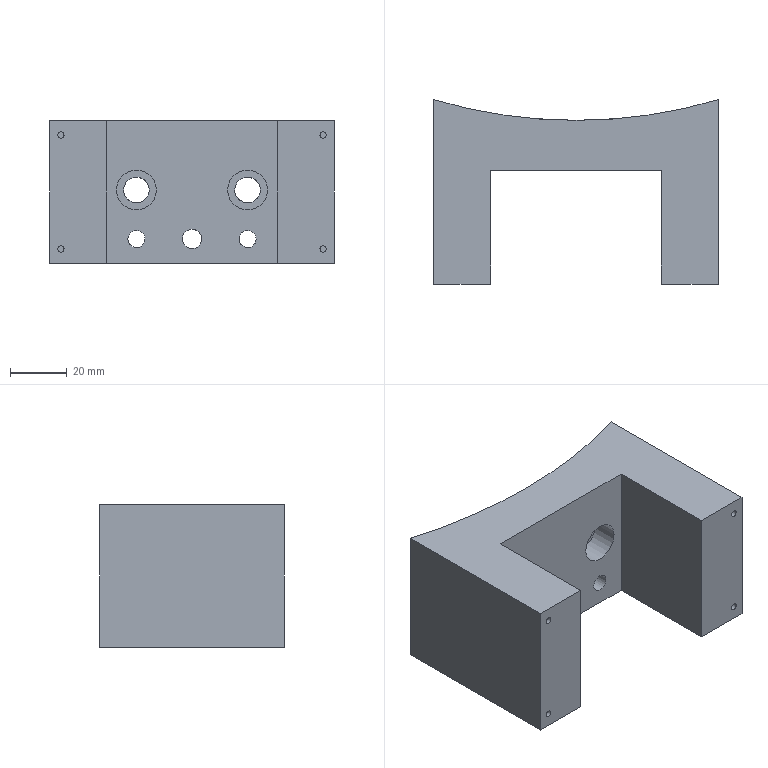NC program | NX | posted with a generic post | part box 100 x 64.77 x 50 mm
Lines 1 to 978 of 7818:
N10 G17 G21 G94 G90
(ZLEVEL_PROFILE_1 , TOOL : D50R0.8)
N12 T02 M6
N14 G54
N16 G17 G0 G90 X2.648 Y76.918 B0. C0. S1200 M3
N18 G43 Z30. H2
N20 Z7.002
N22 G94 G1 X2.631 Y76.907 Z6.512 F1500.
N24 X2.581 Y76.87 Z6.043
N26 X2.501 Y76.808 Z5.594
N28 X2.391 Y76.72 Z5.164
N30 X2.254 Y76.602 Z4.754
N32 X2.093 Y76.455 Z4.363
N34 X1.908 Y76.278 Z3.99
N36 X1.702 Y76.068 Z3.636
N38 X1.476 Y75.825 Z3.299
N40 X1.234 Y75.547 Z2.979
N42 X0.976 Y75.233 Z2.677
N44 X0.704 Y74.881 Z2.391
N46 X0.421 Y74.492 Z2.121
N48 X0.128 Y74.062 Z1.867
N50 X-0.173 Y73.591 Z1.629
N52 X-0.479 Y73.078 Z1.405
N54 X-0.789 Y72.52 Z1.196
N56 X-1.102 Y71.918 Z1.002
N58 X-1.414 Y71.27 Z0.821
N60 X-1.724 Y70.574 Z0.654
N62 X-2.03 Y69.829 Z0.5
N64 X-2.331 Y69.034 Z0.359
N66 X-2.624 Y68.188 Z0.23
N68 X-2.907 Y67.289 Z0.113
N70 X-3.179 Y66.336 Z0.008
N72 X-3.437 Y65.327 Z-0.087
N74 X-3.679 Y64.262 Z-0.17
N76 X-3.905 Y63.139 Z-0.243
N78 X-4.111 Y61.957 Z-0.306
N80 X-4.296 Y60.715 Z-0.359
N82 X-4.457 Y59.41 Z-0.403
N84 X-4.594 Y58.043 Z-0.438
N86 X-4.704 Y56.612 Z-0.465
N88 X-4.784 Y55.115 Z-0.484
N90 X-4.834 Y53.551 Z-0.495
N92 X-4.851 Y51.918 Z-0.498
N94 X-4.85 Y22.992
N96 Y-25.
N98 X-4.851 Y-51.918
N100 X-4.835 Y-52.334
N102 X-4.788 Y-52.725
N104 X-4.714 Y-53.093
N106 X-4.613 Y-53.437
N108 X-4.488 Y-53.759
N110 X-4.341 Y-54.06
N112 X-4.175 Y-54.34
N114 X-3.991 Y-54.6
N116 X-3.792 Y-54.841
N118 X-3.58 Y-55.064
N120 X-3.358 Y-55.268
N122 X-3.127 Y-55.456
N124 X-2.889 Y-55.627
N126 X-2.648 Y-55.782
N128 X-2.404 Y-55.923
N130 X-2.161 Y-56.05
N132 X-1.92 Y-56.163
N134 X-1.52 Y-56.327
N136 X-1.13 Y-56.455
N138 X-0.749 Y-56.546
N140 X-0.373 Y-56.6
N142 X0.001 Y-56.618
N144 X0.374 Y-56.6
N146 X0.75 Y-56.546
N148 X1.132 Y-56.455
N150 X1.521 Y-56.327
N152 X1.921 Y-56.163
N154 X2.162 Y-56.05
N156 X2.405 Y-55.923
N158 X2.649 Y-55.782
N160 X2.891 Y-55.627
N162 X3.128 Y-55.456
N164 X3.359 Y-55.268
N166 X3.582 Y-55.064
N168 X3.793 Y-54.841
N170 X3.992 Y-54.6
N172 X4.176 Y-54.34
N174 X4.342 Y-54.06
N176 X4.489 Y-53.759
N178 X4.614 Y-53.437
N180 X4.715 Y-53.093
N182 X4.79 Y-52.725
N184 X4.836 Y-52.334
N186 X4.852 Y-51.918
N188 Y-25.76
N190 X4.85 Y-25.006
N192 Y22.992
N194 X4.852 Y51.918
N196 X4.836 Y52.335 Z-0.499
N198 X4.79 Y52.726 Z-0.501
N200 X4.715 Y53.094 Z-0.504
N202 X4.614 Y53.439 Z-0.508
N204 X4.489 Y53.762 Z-0.513
N206 X4.342 Y54.063 Z-0.519
N208 X4.176 Y54.344 Z-0.526
N210 X3.992 Y54.604 Z-0.534
N212 X3.793 Y54.846 Z-0.543
N214 X3.581 Y55.068 Z-0.552
N216 X3.359 Y55.273 Z-0.562
N218 X3.128 Y55.461 Z-0.573
N220 X2.89 Y55.633 Z-0.584
N222 X2.649 Y55.789 Z-0.596
N224 X2.405 Y55.93 Z-0.608
N226 X2.162 Y56.057 Z-0.62
N228 X1.921 Y56.171 Z-0.633
N230 X1.521 Y56.335 Z-0.655
N232 X1.131 Y56.463 Z-0.678
N234 X0.75 Y56.555 Z-0.701
N236 X0.374 Y56.61 Z-0.724
N238 X0.001 Y56.628 Z-0.747
N240 X-0.373 Y56.61 Z-0.771
N242 X-0.749 Y56.556 Z-0.794
N244 X-1.13 Y56.465 Z-0.817
N246 X-1.519 Y56.338 Z-0.839
N248 X-1.919 Y56.174 Z-0.861
N250 X-2.16 Y56.061 Z-0.874
N252 X-2.404 Y55.934 Z-0.886
N254 X-2.647 Y55.793 Z-0.899
N256 X-2.889 Y55.638 Z-0.91
N258 X-3.127 Y55.466 Z-0.921
N260 X-3.358 Y55.279 Z-0.932
N262 X-3.58 Y55.074 Z-0.942
N264 X-3.792 Y54.852 Z-0.952
N266 X-3.991 Y54.611 Z-0.96
N268 X-4.174 Y54.35 Z-0.968
N270 X-4.341 Y54.07 Z-0.975
N272 X-4.488 Y53.769 Z-0.981
N274 X-4.612 Y53.446 Z-0.987
N276 X-4.714 Y53.101 Z-0.991
N278 X-4.788 Y52.734 Z-0.994
N280 X-4.835 Y52.342 Z-0.996
N282 X-4.851 Y51.926
N284 X-4.85 Y24.701
N286 Y-25.
N288 X-4.851 Y-51.926
N290 X-4.835 Y-52.341
N292 X-4.788 Y-52.732
N294 X-4.713 Y-53.1
N296 X-4.612 Y-53.444
N298 X-4.487 Y-53.767
N300 X-4.34 Y-54.068
N302 X-4.174 Y-54.348
N304 X-3.99 Y-54.608
N306 X-3.791 Y-54.849
N308 X-3.579 Y-55.071
N310 X-3.356 Y-55.275
N312 X-3.125 Y-55.463
N314 X-2.887 Y-55.634
N316 X-2.645 Y-55.79
N318 X-2.401 Y-55.931
N320 X-2.157 Y-56.057
N322 X-1.916 Y-56.171
N324 X-1.515 Y-56.335
N326 X-1.125 Y-56.462
N328 X-0.743 Y-56.553
N330 X-0.367 Y-56.607
N332 X0.007 Y-56.626
N334 X0.381 Y-56.607
N336 X0.758 Y-56.553
N338 X1.14 Y-56.462
N340 X1.529 Y-56.335
N342 X1.93 Y-56.171
N344 X2.171 Y-56.057
N346 X2.414 Y-55.931
N348 X2.657 Y-55.79
N350 X2.899 Y-55.634
N352 X3.136 Y-55.463
N354 X3.367 Y-55.275
N356 X3.589 Y-55.071
N358 X3.801 Y-54.849
N360 X3.999 Y-54.608
N362 X4.182 Y-54.348
N364 X4.348 Y-54.068
N366 X4.494 Y-53.767
N368 X4.618 Y-53.444
N370 X4.718 Y-53.1
N372 X4.792 Y-52.732
N374 X4.837 Y-52.341
N376 X4.852 Y-51.926
N378 X4.851 Y-51.519
N380 Y-26.035
N382 X4.85 Y-25.
N384 Y24.701
N386 X4.852 Y51.926
N388 X4.836 Y52.342 Z-0.997
N390 X4.79 Y52.734 Z-0.999
N392 X4.715 Y53.102 Z-1.002
N394 X4.614 Y53.447 Z-1.006
N396 X4.489 Y53.769 Z-1.011
N398 X4.342 Y54.071 Z-1.017
N400 X4.176 Y54.351 Z-1.024
N402 X3.992 Y54.612 Z-1.032
N404 X3.793 Y54.853 Z-1.041
N406 X3.581 Y55.076 Z-1.05
N408 X3.359 Y55.281 Z-1.06
N410 X3.128 Y55.469 Z-1.071
N412 X2.89 Y55.64 Z-1.082
N414 X2.649 Y55.796 Z-1.094
N416 X2.405 Y55.937 Z-1.106
N418 X2.162 Y56.065 Z-1.118
N420 X1.921 Y56.178 Z-1.131
N422 X1.521 Y56.343 Z-1.153
N424 X1.131 Y56.47 Z-1.176
N426 X0.75 Y56.562 Z-1.199
N428 X0.374 Y56.617 Z-1.222
N430 X0.001 Y56.635 Z-1.245
N432 X-0.373 Y56.618 Z-1.269
N434 X-0.749 Y56.563 Z-1.292
N436 X-1.13 Y56.473 Z-1.315
N438 X-1.519 Y56.345 Z-1.337
N440 X-1.919 Y56.182 Z-1.359
N442 X-2.16 Y56.068 Z-1.372
N444 X-2.404 Y55.942 Z-1.385
N446 X-2.647 Y55.801 Z-1.397
N448 X-2.889 Y55.645 Z-1.408
N450 X-3.127 Y55.474 Z-1.42
N452 X-3.358 Y55.286 Z-1.43
N454 X-3.58 Y55.082 Z-1.44
N456 X-3.792 Y54.859 Z-1.45
N458 X-3.991 Y54.618 Z-1.458
N460 X-4.174 Y54.358 Z-1.466
N462 X-4.341 Y54.077 Z-1.473
N464 X-4.488 Y53.776 Z-1.48
N466 X-4.613 Y53.454 Z-1.485
N468 X-4.714 Y53.109 Z-1.489
N470 X-4.788 Y52.741 Z-1.492
N472 X-4.835 Y52.349 Z-1.494
N474 X-4.851 Y51.933
N476 X-4.85 Y24.701
N478 Y-25.
N480 X-4.851 Y-51.933
N482 X-4.835 Y-52.349
N484 X-4.788 Y-52.74
N486 X-4.713 Y-53.107
N488 X-4.612 Y-53.452
N490 X-4.487 Y-53.774
N492 X-4.34 Y-54.075
N494 X-4.174 Y-54.355
N496 X-3.99 Y-54.615
N498 X-3.791 Y-54.856
N500 X-3.579 Y-55.078
N502 X-3.356 Y-55.283
N504 X-3.125 Y-55.47
N506 X-2.887 Y-55.641
N508 X-2.645 Y-55.797
N510 X-2.401 Y-55.938
N512 X-2.157 Y-56.065
N514 X-1.916 Y-56.178
N516 X-1.515 Y-56.342
N518 X-1.125 Y-56.469
N520 X-0.743 Y-56.56
N522 X-0.367 Y-56.615
N524 X0.007 Y-56.633
N526 X0.381 Y-56.615
N528 X0.758 Y-56.56
N530 X1.14 Y-56.469
N532 X1.529 Y-56.342
N534 X1.93 Y-56.178
N536 X2.171 Y-56.065
N538 X2.414 Y-55.938
N540 X2.657 Y-55.797
N542 X2.899 Y-55.641
N544 X3.136 Y-55.47
N546 X3.367 Y-55.283
N548 X3.589 Y-55.078
N550 X3.801 Y-54.856
N552 X3.999 Y-54.615
N554 X4.182 Y-54.355
N556 X4.348 Y-54.075
N558 X4.494 Y-53.774
N560 X4.618 Y-53.452
N562 X4.718 Y-53.107
N564 X4.792 Y-52.74
N566 X4.837 Y-52.349
N568 X4.852 Y-51.933
N570 X4.851 Y-51.519
N572 Y-26.035
N574 X4.85 Y-25.
N576 Y24.701
N578 X4.852 Y51.933
N580 X4.836 Y52.349 Z-1.495
N582 X4.79 Y52.741 Z-1.497
N584 X4.715 Y53.109 Z-1.5
N586 X4.614 Y53.454 Z-1.504
N588 X4.489 Y53.777 Z-1.509
N590 X4.342 Y54.078 Z-1.515
N592 X4.176 Y54.359 Z-1.522
N594 X3.992 Y54.619 Z-1.53
N596 X3.793 Y54.86 Z-1.539
N598 X3.581 Y55.083 Z-1.548
N600 X3.359 Y55.288 Z-1.559
N602 X3.128 Y55.476 Z-1.569
N604 X2.89 Y55.648 Z-1.58
N606 X2.649 Y55.804 Z-1.592
N608 X2.405 Y55.945 Z-1.604
N610 X2.162 Y56.072 Z-1.617
N612 X1.921 Y56.186 Z-1.629
N614 X1.521 Y56.35 Z-1.651
N616 X1.131 Y56.478 Z-1.674
N618 X0.75 Y56.569 Z-1.697
N620 X0.374 Y56.624 Z-1.72
N622 X0.001 Y56.643 Z-1.743
N624 X-0.373 Y56.625 Z-1.767
N626 X-0.749 Y56.571 Z-1.79
N628 X-1.13 Y56.48 Z-1.813
N630 X-1.519 Y56.353 Z-1.836
N632 X-1.919 Y56.189 Z-1.858
N634 X-2.16 Y56.076 Z-1.87
N636 X-2.404 Y55.949 Z-1.883
N638 X-2.647 Y55.808 Z-1.895
N640 X-2.889 Y55.652 Z-1.906
N642 X-3.127 Y55.481 Z-1.918
N644 X-3.358 Y55.294 Z-1.928
N646 X-3.58 Y55.089 Z-1.938
N648 X-3.792 Y54.866 Z-1.948
N650 X-3.991 Y54.625 Z-1.957
N652 X-4.174 Y54.365 Z-1.964
N654 X-4.341 Y54.085 Z-1.972
N656 X-4.488 Y53.784 Z-1.978
N658 X-4.613 Y53.461 Z-1.983
N660 X-4.714 Y53.116 Z-1.987
N662 X-4.788 Y52.748 Z-1.99
N664 X-4.835 Y52.357 Z-1.992
N666 X-4.851 Y51.94 Z-1.993
N668 X-4.85 Y24.701
N670 Y-25.
N672 X-4.851 Y-51.94
N674 X-4.835 Y-52.356
N676 X-4.788 Y-52.747
N678 X-4.713 Y-53.115
N680 X-4.612 Y-53.459
N682 X-4.487 Y-53.781
N684 X-4.34 Y-54.082
N686 X-4.174 Y-54.362
N688 X-3.99 Y-54.622
N690 X-3.791 Y-54.863
N692 X-3.579 Y-55.086
N694 X-3.356 Y-55.29
N696 X-3.125 Y-55.478
N698 X-2.887 Y-55.649
N700 X-2.645 Y-55.804
N702 X-2.401 Y-55.945
N704 X-2.157 Y-56.072
N706 X-1.916 Y-56.185
N708 X-1.515 Y-56.349
N710 X-1.125 Y-56.477
N712 X-0.743 Y-56.568
N714 X-0.367 Y-56.622
N716 X0.007 Y-56.64
N718 X0.381 Y-56.622
N720 X0.758 Y-56.567
N722 X1.14 Y-56.477
N724 X1.529 Y-56.349
N726 X1.93 Y-56.185
N728 X2.171 Y-56.072
N730 X2.414 Y-55.945
N732 X2.657 Y-55.804
N734 X2.899 Y-55.649
N736 X3.136 Y-55.478
N738 X3.367 Y-55.29
N740 X3.589 Y-55.085
N742 X3.801 Y-54.863
N744 X3.999 Y-54.622
N746 X4.182 Y-54.362
N748 X4.348 Y-54.082
N750 X4.494 Y-53.781
N752 X4.618 Y-53.459
N754 X4.718 Y-53.115
N756 X4.792 Y-52.747
N758 X4.837 Y-52.356
N760 X4.852 Y-51.94
N762 X4.851 Y-51.519
N764 Y-26.035
N766 X4.85 Y-25.
N768 Y24.701
N770 X4.852 Y51.94
N772 X4.836 Y52.356
N774 X4.79 Y52.748 Z-1.995
N776 X4.715 Y53.116 Z-1.998
N778 X4.614 Y53.461 Z-2.002
N780 X4.489 Y53.784 Z-2.007
N782 X4.342 Y54.085 Z-2.013
N784 X4.176 Y54.366 Z-2.021
N786 X3.992 Y54.626 Z-2.028
N788 X3.793 Y54.868 Z-2.037
N790 X3.581 Y55.09 Z-2.047
N792 X3.359 Y55.295 Z-2.057
N794 X3.128 Y55.483 Z-2.067
N796 X2.89 Y55.655 Z-2.079
N798 X2.649 Y55.811 Z-2.09
N800 X2.405 Y55.952 Z-2.102
N802 X2.162 Y56.079 Z-2.115
N804 X1.921 Y56.193 Z-2.127
N806 X1.521 Y56.357 Z-2.149
N808 X1.131 Y56.485 Z-2.172
N810 X0.75 Y56.577 Z-2.195
N812 X0.374 Y56.632 Z-2.218
N814 X0.001 Y56.65 Z-2.242
N816 X-0.373 Y56.632 Z-2.265
N818 X-0.749 Y56.578 Z-2.288
N820 X-1.13 Y56.487 Z-2.311
N822 X-1.519 Y56.36 Z-2.334
N824 X-1.919 Y56.196 Z-2.356
N826 X-2.16 Y56.083 Z-2.368
N828 X-2.404 Y55.956 Z-2.381
N830 X-2.647 Y55.815 Z-2.393
N832 X-2.889 Y55.66 Z-2.405
N834 X-3.127 Y55.488 Z-2.416
N836 X-3.358 Y55.301 Z-2.426
N838 X-3.58 Y55.096 Z-2.437
N840 X-3.792 Y54.874 Z-2.446
N842 X-3.991 Y54.633 Z-2.455
N844 X-4.174 Y54.372 Z-2.463
N846 X-4.341 Y54.092 Z-2.47
N848 X-4.488 Y53.791 Z-2.476
N850 X-4.613 Y53.468 Z-2.481
N852 X-4.714 Y53.123 Z-2.485
N854 X-4.788 Y52.755 Z-2.488
N856 X-4.835 Y52.364 Z-2.49
N858 X-4.851 Y51.948 Z-2.491
N860 X-4.85 Y24.701
N862 Y-25.
N864 X-4.851 Y-51.948
N866 X-4.835 Y-52.363
N868 X-4.788 Y-52.754
N870 X-4.713 Y-53.122
N872 X-4.612 Y-53.466
N874 X-4.487 Y-53.789
N876 X-4.34 Y-54.09
N878 X-4.174 Y-54.37
N880 X-3.99 Y-54.63
N882 X-3.791 Y-54.871
N884 X-3.579 Y-55.093
N886 X-3.356 Y-55.297
N888 X-3.125 Y-55.485
N890 X-2.887 Y-55.656
N892 X-2.645 Y-55.812
N894 X-2.401 Y-55.953
N896 X-2.157 Y-56.079
N898 X-1.916 Y-56.193
N900 X-1.515 Y-56.357
N902 X-1.125 Y-56.484
N904 X-0.743 Y-56.575
N906 X-0.367 Y-56.629
N908 X0.007 Y-56.648
N910 X0.381 Y-56.629
N912 X0.758 Y-56.575
N914 X1.14 Y-56.484
N916 X1.529 Y-56.356
N918 X1.93 Y-56.193
N920 X2.171 Y-56.079
N922 X2.414 Y-55.953
N924 X2.657 Y-55.812
N926 X2.899 Y-55.656
N928 X3.136 Y-55.485
N930 X3.367 Y-55.297
N932 X3.589 Y-55.093
N934 X3.801 Y-54.87
N936 X3.999 Y-54.63
N938 X4.182 Y-54.37
N940 X4.348 Y-54.089
N942 X4.494 Y-53.789
N944 X4.618 Y-53.466
N946 X4.718 Y-53.122
N948 X4.792 Y-52.754
N950 X4.837 Y-52.363
N952 X4.852 Y-51.948
N954 X4.851 Y-51.519
N956 Y-26.035
N958 X4.85 Y-25.
N960 Y24.701
N962 X4.852 Y51.948
N964 X4.836 Y52.364
N966 X4.79 Y52.756 Z-2.493
N968 X4.715 Y53.124 Z-2.496
N970 X4.614 Y53.469 Z-2.5
N972 X4.489 Y53.791 Z-2.505
N974 X4.342 Y54.093 Z-2.512
N976 X4.176 Y54.373 Z-2.519
N978 X3.992 Y54.634 Z-2.527
N980 X3.793 Y54.875 Z-2.535
N982 X3.581 Y55.098 Z-2.545
N984 X3.359 Y55.303 Z-2.555
N986 X3.128 Y55.491 Z-2.565
N988 X2.89 Y55.662 Z-2.577
N990 X2.649 Y55.818 Z-2.588
N992 X2.405 Y55.959 Z-2.6
N994 X2.162 Y56.087 Z-2.613
N996 X1.921 Y56.2 Z-2.626
N998 X1.521 Y56.365 Z-2.648
N1000 X1.131 Y56.492 Z-2.67
N1002 X0.75 Y56.584 Z-2.693
N1004 X0.374 Y56.639 Z-2.716
N1006 X0.001 Y56.657 Z-2.74
N1008 X-0.373 Y56.64 Z-2.763
N1010 X-0.749 Y56.585 Z-2.786
N1012 X-1.13 Y56.495 Z-2.809
N1014 X-1.519 Y56.367 Z-2.832
N1016 X-1.92 Y56.204 Z-2.854
N1018 X-2.16 Y56.09 Z-2.867
N1020 X-2.404 Y55.964 Z-2.879
N1022 X-2.647 Y55.823 Z-2.891
N1024 X-2.889 Y55.667 Z-2.903
N1026 X-3.127 Y55.496 Z-2.914
N1028 X-3.358 Y55.308 Z-2.925
N1030 X-3.58 Y55.103 Z-2.935
N1032 X-3.792 Y54.881 Z-2.944
N1034 X-3.991 Y54.64 Z-2.953
N1036 X-4.175 Y54.38 Z-2.961
N1038 X-4.341 Y54.099 Z-2.968
N1040 X-4.488 Y53.798 Z-2.974
N1042 X-4.613 Y53.476 Z-2.979
N1044 X-4.714 Y53.131 Z-2.983
N1046 X-4.789 Y52.763 Z-2.986
N1048 X-4.835 Y52.371 Z-2.988
N1050 X-4.851 Y51.955 Z-2.989
N1052 X-4.85 Y24.701
N1054 Y-25.
N1056 X-4.851 Y-51.955
N1058 X-4.835 Y-52.371
N1060 X-4.788 Y-52.762
N1062 X-4.713 Y-53.129
N1064 X-4.612 Y-53.474
N1066 X-4.487 Y-53.796
N1068 X-4.34 Y-54.097
N1070 X-4.174 Y-54.377
N1072 X-3.99 Y-54.637
N1074 X-3.791 Y-54.878
N1076 X-3.579 Y-55.1
N1078 X-3.356 Y-55.305
N1080 X-3.125 Y-55.492
N1082 X-2.887 Y-55.663
N1084 X-2.645 Y-55.819
N1086 X-2.401 Y-55.96
N1088 X-2.157 Y-56.087
N1090 X-1.916 Y-56.2
N1092 X-1.515 Y-56.364
N1094 X-1.125 Y-56.491
N1096 X-0.743 Y-56.582
N1098 X-0.367 Y-56.637
N1100 X0.007 Y-56.655
N1102 X0.381 Y-56.637
N1104 X0.758 Y-56.582
N1106 X1.14 Y-56.491
N1108 X1.529 Y-56.364
N1110 X1.93 Y-56.2
N1112 X2.171 Y-56.087
N1114 X2.414 Y-55.96
N1116 X2.657 Y-55.819
N1118 X2.899 Y-55.663
N1120 X3.136 Y-55.492
N1122 X3.367 Y-55.305
N1124 X3.589 Y-55.1
N1126 X3.801 Y-54.878
N1128 X3.999 Y-54.637
N1130 X4.182 Y-54.377
N1132 X4.348 Y-54.097
N1134 X4.494 Y-53.796
N1136 X4.618 Y-53.474
N1138 X4.718 Y-53.129
N1140 X4.792 Y-52.762
N1142 X4.837 Y-52.371
N1144 X4.852 Y-51.955
N1146 X4.851 Y-51.519
N1148 Y-26.035
N1150 X4.85 Y-25.
N1152 Y24.701
N1154 X4.852 Y51.955
N1156 X4.836 Y52.371
N1158 X4.79 Y52.763 Z-2.991
N1160 X4.715 Y53.131 Z-2.994
N1162 X4.614 Y53.476 Z-2.998
N1164 X4.489 Y53.799 Z-3.004
N1166 X4.342 Y54.1 Z-3.01
N1168 X4.176 Y54.38 Z-3.017
N1170 X3.992 Y54.641 Z-3.025
N1172 X3.793 Y54.882 Z-3.033
N1174 X3.581 Y55.105 Z-3.043
N1176 X3.359 Y55.31 Z-3.053
N1178 X3.128 Y55.498 Z-3.064
N1180 X2.89 Y55.67 Z-3.075
N1182 X2.649 Y55.826 Z-3.086
N1184 X2.405 Y55.967 Z-3.099
N1186 X2.162 Y56.094 Z-3.111
N1188 X1.921 Y56.208 Z-3.124
N1190 X1.521 Y56.372 Z-3.146
N1192 X1.131 Y56.5 Z-3.168
N1194 X0.75 Y56.591 Z-3.191
N1196 X0.374 Y56.646 Z-3.214
N1198 X0.001 Y56.665 Z-3.238
N1200 X-0.373 Y56.647 Z-3.261
N1202 X-0.749 Y56.593 Z-3.284
N1204 X-1.13 Y56.502 Z-3.307
N1206 X-1.519 Y56.375 Z-3.33
N1208 X-1.92 Y56.211 Z-3.352
N1210 X-2.16 Y56.098 Z-3.365
N1212 X-2.404 Y55.971 Z-3.377
N1214 X-2.647 Y55.83 Z-3.389
N1216 X-2.889 Y55.674 Z-3.401
N1218 X-3.127 Y55.503 Z-3.412
N1220 X-3.358 Y55.315 Z-3.423
N1222 X-3.58 Y55.111 Z-3.433
N1224 X-3.792 Y54.888 Z-3.442
N1226 X-3.991 Y54.647 Z-3.451
N1228 X-4.175 Y54.387 Z-3.459
N1230 X-4.341 Y54.107 Z-3.466
N1232 X-4.488 Y53.806 Z-3.472
N1234 X-4.613 Y53.483 Z-3.477
N1236 X-4.714 Y53.138 Z-3.481
N1238 X-4.789 Y52.77 Z-3.484
N1240 X-4.835 Y52.378 Z-3.486
N1242 X-4.851 Y51.962 Z-3.487
N1244 X-4.85 Y24.701
N1246 Y-25.
N1248 X-4.851 Y-51.962
N1250 X-4.835 Y-52.378
N1252 X-4.788 Y-52.769
N1254 X-4.714 Y-53.137
N1256 X-4.612 Y-53.481
N1258 X-4.487 Y-53.803
N1260 X-4.34 Y-54.104
N1262 X-4.174 Y-54.384
N1264 X-3.99 Y-54.644
N1266 X-3.791 Y-54.885
N1268 X-3.579 Y-55.107
N1270 X-3.356 Y-55.312
N1272 X-3.125 Y-55.5
N1274 X-2.887 Y-55.671
N1276 X-2.645 Y-55.826
N1278 X-2.401 Y-55.967
N1280 X-2.157 Y-56.094
N1282 X-1.916 Y-56.207
N1284 X-1.515 Y-56.371
N1286 X-1.125 Y-56.499
N1288 X-0.743 Y-56.589
N1290 X-0.367 Y-56.644
N1292 X0.007 Y-56.662
N1294 X0.381 Y-56.644
N1296 X0.758 Y-56.589
N1298 X1.14 Y-56.498
N1300 X1.529 Y-56.371
N1302 X1.93 Y-56.207
N1304 X2.171 Y-56.094
N1306 X2.414 Y-55.967
N1308 X2.657 Y-55.826
N1310 X2.899 Y-55.671
N1312 X3.136 Y-55.499
N1314 X3.367 Y-55.312
N1316 X3.589 Y-55.107
N1318 X3.801 Y-54.885
N1320 X3.999 Y-54.644
N1322 X4.182 Y-54.384
N1324 X4.348 Y-54.104
N1326 X4.494 Y-53.803
N1328 X4.618 Y-53.481
N1330 X4.718 Y-53.136
N1332 X4.792 Y-52.769
N1334 X4.837 Y-52.378
N1336 X4.852 Y-51.962
N1338 X4.851 Y-51.519
N1340 Y-26.035
N1342 X4.85 Y-25.
N1344 Y24.701
N1346 X4.852 Y51.962
N1348 X4.836 Y52.378 Z-3.488
N1350 X4.79 Y52.77 Z-3.489
N1352 X4.715 Y53.138 Z-3.492
N1354 X4.614 Y53.483 Z-3.497
N1356 X4.489 Y53.806 Z-3.502
N1358 X4.342 Y54.107 Z-3.508
N1360 X4.176 Y54.388 Z-3.515
N1362 X3.992 Y54.648 Z-3.523
N1364 X3.793 Y54.89 Z-3.532
N1366 X3.581 Y55.112 Z-3.541
N1368 X3.359 Y55.317 Z-3.551
N1370 X3.128 Y55.505 Z-3.562
N1372 X2.89 Y55.677 Z-3.573
N1374 X2.649 Y55.833 Z-3.585
N1376 X2.405 Y55.974 Z-3.597
N1378 X2.162 Y56.101 Z-3.609
N1380 X1.921 Y56.215 Z-3.622
N1382 X1.521 Y56.379 Z-3.644
N1384 X1.131 Y56.507 Z-3.666
N1386 X0.75 Y56.599 Z-3.689
N1388 X0.374 Y56.654 Z-3.713
N1390 X0.001 Y56.672 Z-3.736
N1392 X-0.373 Y56.654 Z-3.759
N1394 X-0.749 Y56.6 Z-3.782
N1396 X-1.13 Y56.509 Z-3.805
N1398 X-1.519 Y56.382 Z-3.828
N1400 X-1.92 Y56.218 Z-3.85
N1402 X-2.16 Y56.105 Z-3.863
N1404 X-2.404 Y55.978 Z-3.875
N1406 X-2.647 Y55.837 Z-3.887
N1408 X-2.889 Y55.682 Z-3.899
N1410 X-3.127 Y55.51 Z-3.91
N1412 X-3.358 Y55.323 Z-3.921
N1414 X-3.58 Y55.118 Z-3.931
N1416 X-3.792 Y54.896 Z-3.94
N1418 X-3.991 Y54.655 Z-3.949
N1420 X-4.175 Y54.394 Z-3.957
N1422 X-4.341 Y54.114 Z-3.964
N1424 X-4.488 Y53.813 Z-3.97
N1426 X-4.613 Y53.49 Z-3.975
N1428 X-4.714 Y53.145 Z-3.979
N1430 X-4.789 Y52.777 Z-3.983
N1432 X-4.835 Y52.386 Z-3.984
N1434 X-4.851 Y51.97 Z-3.985
N1436 X-4.85 Y24.701
N1438 Y-25.
N1440 X-4.851 Y-51.97
N1442 X-4.835 Y-52.385
N1444 X-4.788 Y-52.776
N1446 X-4.714 Y-53.144
N1448 X-4.612 Y-53.488
N1450 X-4.487 Y-53.811
N1452 X-4.34 Y-54.111
N1454 X-4.174 Y-54.392
N1456 X-3.99 Y-54.652
N1458 X-3.791 Y-54.892
N1460 X-3.579 Y-55.115
N1462 X-3.356 Y-55.319
N1464 X-3.125 Y-55.507
N1466 X-2.887 Y-55.678
N1468 X-2.645 Y-55.834
N1470 X-2.401 Y-55.975
N1472 X-2.157 Y-56.101
N1474 X-1.916 Y-56.215
N1476 X-1.515 Y-56.378
N1478 X-1.125 Y-56.506
N1480 X-0.743 Y-56.597
N1482 X-0.367 Y-56.651
N1484 X0.007 Y-56.67
N1486 X0.381 Y-56.651
N1488 X0.758 Y-56.597
N1490 X1.14 Y-56.506
N1492 X1.529 Y-56.378
N1494 X1.93 Y-56.215
N1496 X2.171 Y-56.101
N1498 X2.414 Y-55.974
N1500 X2.657 Y-55.834
N1502 X2.899 Y-55.678
N1504 X3.136 Y-55.507
N1506 X3.367 Y-55.319
N1508 X3.589 Y-55.115
N1510 X3.801 Y-54.892
N1512 X3.999 Y-54.652
N1514 X4.182 Y-54.392
N1516 X4.348 Y-54.111
N1518 X4.494 Y-53.811
N1520 X4.618 Y-53.488
N1522 X4.718 Y-53.144
N1524 X4.792 Y-52.776
N1526 X4.837 Y-52.385
N1528 X4.852 Y-51.97
N1530 X4.851 Y-51.519
N1532 Y-26.035
N1534 X4.85 Y-25.
N1536 Y24.701
N1538 X4.852 Y51.97
N1540 X4.836 Y52.386 Z-3.986
N1542 X4.79 Y52.777 Z-3.988
N1544 X4.715 Y53.145 Z-3.991
N1546 X4.614 Y53.49 Z-3.995
N1548 X4.489 Y53.813 Z-4.
N1550 X4.342 Y54.115 Z-4.006
N1552 X4.176 Y54.395 Z-4.013
N1554 X3.992 Y54.656 Z-4.021
N1556 X3.793 Y54.897 Z-4.03
N1558 X3.581 Y55.12 Z-4.039
N1560 X3.359 Y55.325 Z-4.049
N1562 X3.128 Y55.513 Z-4.06
N1564 X2.89 Y55.684 Z-4.071
N1566 X2.649 Y55.84 Z-4.083
N1568 X2.405 Y55.981 Z-4.095
N1570 X2.162 Y56.109 Z-4.107
N1572 X1.921 Y56.222 Z-4.12
N1574 X1.521 Y56.387 Z-4.142
N1576 X1.131 Y56.514 Z-4.165
N1578 X0.75 Y56.606 Z-4.188
N1580 X0.374 Y56.661 Z-4.211
N1582 X0.001 Y56.679 Z-4.234
N1584 X-0.373 Y56.662 Z-4.257
N1586 X-0.749 Y56.607 Z-4.281
N1588 X-1.13 Y56.516 Z-4.304
N1590 X-1.519 Y56.389 Z-4.326
N1592 X-1.92 Y56.226 Z-4.348
N1594 X-2.16 Y56.112 Z-4.361
N1596 X-2.404 Y55.985 Z-4.373
N1598 X-2.647 Y55.845 Z-4.385
N1600 X-2.889 Y55.689 Z-4.397
N1602 X-3.127 Y55.518 Z-4.408
N1604 X-3.358 Y55.33 Z-4.419
N1606 X-3.58 Y55.125 Z-4.429
N1608 X-3.792 Y54.903 Z-4.438
N1610 X-3.991 Y54.662 Z-4.447
N1612 X-4.175 Y54.402 Z-4.455
N1614 X-4.341 Y54.121 Z-4.462
N1616 X-4.488 Y53.82 Z-4.468
N1618 X-4.613 Y53.498 Z-4.473
N1620 X-4.714 Y53.153 Z-4.478
N1622 X-4.789 Y52.785 Z-4.481
N1624 X-4.835 Y52.393 Z-4.482
N1626 X-4.851 Y51.977 Z-4.483
N1628 X-4.85 Y24.701
N1630 Y-25.
N1632 X-4.851 Y-51.977
N1634 X-4.835 Y-52.392
N1636 X-4.789 Y-52.784
N1638 X-4.714 Y-53.151
N1640 X-4.613 Y-53.496
N1642 X-4.488 Y-53.818
N1644 X-4.341 Y-54.119
N1646 X-4.175 Y-54.399
N1648 X-3.991 Y-54.659
N1650 X-3.792 Y-54.9
N1652 X-3.581 Y-55.122
N1654 X-3.358 Y-55.327
N1656 X-3.127 Y-55.514
N1658 X-2.889 Y-55.685
N1660 X-2.648 Y-55.841
N1662 X-2.404 Y-55.982
N1664 X-2.161 Y-56.109
N1666 X-1.92 Y-56.222
N1668 X-1.52 Y-56.386
N1670 X-1.13 Y-56.513
N1672 X-0.749 Y-56.604
N1674 X-0.373 Y-56.659
N1676 X0.001 Y-56.677
N1678 X0.374 Y-56.659
N1680 X0.75 Y-56.604
N1682 X1.132 Y-56.513
N1684 X1.521 Y-56.386
N1686 X1.921 Y-56.222
N1688 X2.162 Y-56.109
N1690 X2.406 Y-55.982
N1692 X2.649 Y-55.841
N1694 X2.891 Y-55.685
N1696 X3.128 Y-55.514
N1698 X3.359 Y-55.327
N1700 X3.582 Y-55.122
N1702 X3.794 Y-54.9
N1704 X3.992 Y-54.659
N1706 X4.176 Y-54.399
N1708 X4.342 Y-54.119
N1710 X4.489 Y-53.818
N1712 X4.614 Y-53.496
N1714 X4.715 Y-53.151
N1716 X4.79 Y-52.784
N1718 X4.836 Y-52.392
N1720 X4.852 Y-51.977
N1722 X4.85 Y-25.
N1724 Y24.701
N1726 X4.852 Y51.977
N1728 X4.836 Y52.393 Z-4.484
N1730 X4.79 Y52.785 Z-4.486
N1732 X4.715 Y53.153 Z-4.489
N1734 X4.614 Y53.498 Z-4.493
N1736 X4.489 Y53.821 Z-4.498
N1738 X4.342 Y54.122 Z-4.504
N1740 X4.176 Y54.402 Z-4.511
N1742 X3.992 Y54.663 Z-4.519
N1744 X3.793 Y54.904 Z-4.528
N1746 X3.581 Y55.127 Z-4.537
N1748 X3.359 Y55.332 Z-4.547
N1750 X3.128 Y55.52 Z-4.558
N1752 X2.89 Y55.691 Z-4.569
N1754 X2.649 Y55.847 Z-4.581
N1756 X2.405 Y55.989 Z-4.593
N1758 X2.162 Y56.116 Z-4.605
N1760 X1.921 Y56.23 Z-4.618
N1762 X1.521 Y56.394 Z-4.64
N1764 X1.131 Y56.522 Z-4.663
N1766 X0.75 Y56.613 Z-4.686
N1768 X0.374 Y56.668 Z-4.709
N1770 X0.001 Y56.687 Z-4.732
N1772 X-0.373 Y56.669 Z-4.756
N1774 X-0.749 Y56.615 Z-4.779
N1776 X-1.13 Y56.524 Z-4.802
N1778 X-1.519 Y56.397 Z-4.824
N1780 X-1.92 Y56.233 Z-4.846
N1782 X-2.161 Y56.12 Z-4.859
N1784 X-2.404 Y55.993 Z-4.871
N1786 X-2.648 Y55.852 Z-4.884
N1788 X-2.889 Y55.696 Z-4.895
N1790 X-3.127 Y55.525 Z-4.906
N1792 X-3.358 Y55.337 Z-4.917
N1794 X-3.58 Y55.133 Z-4.927
N1796 X-3.792 Y54.91 Z-4.937
N1798 X-3.991 Y54.669 Z-4.945
N1800 X-4.175 Y54.409 Z-4.953
N1802 X-4.341 Y54.129 Z-4.96
N1804 X-4.488 Y53.828 Z-4.966
N1806 X-4.613 Y53.505 Z-4.972
N1808 X-4.714 Y53.16 Z-4.976
N1810 X-4.789 Y52.792 Z-4.979
N1812 X-4.835 Y52.4 Z-4.981
N1814 X-4.851 Y51.984
N1816 X-4.85 Y24.701
N1818 Y-25.
N1820 X-4.851 Y-51.984
N1822 X-4.835 Y-52.4
N1824 X-4.789 Y-52.791
N1826 X-4.714 Y-53.158
N1828 X-4.613 Y-53.503
N1830 X-4.488 Y-53.825
N1832 X-4.341 Y-54.126
N1834 X-4.175 Y-54.406
N1836 X-3.991 Y-54.666
N1838 X-3.792 Y-54.907
N1840 X-3.581 Y-55.129
N1842 X-3.358 Y-55.334
N1844 X-3.127 Y-55.521
N1846 X-2.89 Y-55.693
N1848 X-2.648 Y-55.848
N1850 X-2.404 Y-55.989
N1852 X-2.161 Y-56.116
N1854 X-1.92 Y-56.229
N1856 X-1.52 Y-56.393
N1858 X-1.13 Y-56.52
N1860 X-0.749 Y-56.611
N1862 X-0.373 Y-56.666
N1864 X0.001 Y-56.684
N1866 X0.374 Y-56.666
N1868 X0.75 Y-56.611
N1870 X1.132 Y-56.52
N1872 X1.521 Y-56.393
N1874 X1.921 Y-56.229
N1876 X2.162 Y-56.116
N1878 X2.406 Y-55.989
N1880 X2.649 Y-55.848
N1882 X2.891 Y-55.693
N1884 X3.128 Y-55.521
N1886 X3.359 Y-55.334
N1888 X3.582 Y-55.129
N1890 X3.794 Y-54.907
N1892 X3.992 Y-54.666
N1894 X4.176 Y-54.406
N1896 X4.342 Y-54.126
N1898 X4.489 Y-53.825
N1900 X4.614 Y-53.503
N1902 X4.715 Y-53.158
N1904 X4.79 Y-52.791
N1906 X4.836 Y-52.4
N1908 X4.852 Y-51.984
N1910 X4.85 Y-25.
N1912 Y24.701
N1914 X4.852 Y51.984
N1916 X4.836 Y52.4 Z-4.982
N1918 X4.79 Y52.792 Z-4.984
N1920 X4.715 Y53.16 Z-4.987
N1922 X4.614 Y53.505 Z-4.991
N1924 X4.489 Y53.828 Z-4.996
N1926 X4.342 Y54.129 Z-5.002
N1928 X4.176 Y54.41 Z-5.009
N1930 X3.992 Y54.67 Z-5.017
N1932 X3.793 Y54.912 Z-5.026
N1934 X3.581 Y55.134 Z-5.035
N1936 X3.359 Y55.339 Z-5.045
N1938 X3.128 Y55.527 Z-5.056
N1940 X2.89 Y55.699 Z-5.067
N1942 X2.649 Y55.855 Z-5.079
N1944 X2.405 Y55.996 Z-5.091
N1946 X2.162 Y56.123 Z-5.103
N1948 X1.921 Y56.237 Z-5.116
N1950 X1.521 Y56.401 Z-5.138
N1952 X1.131 Y56.529 Z-5.161
N1954 X0.75 Y56.62 Z-5.184